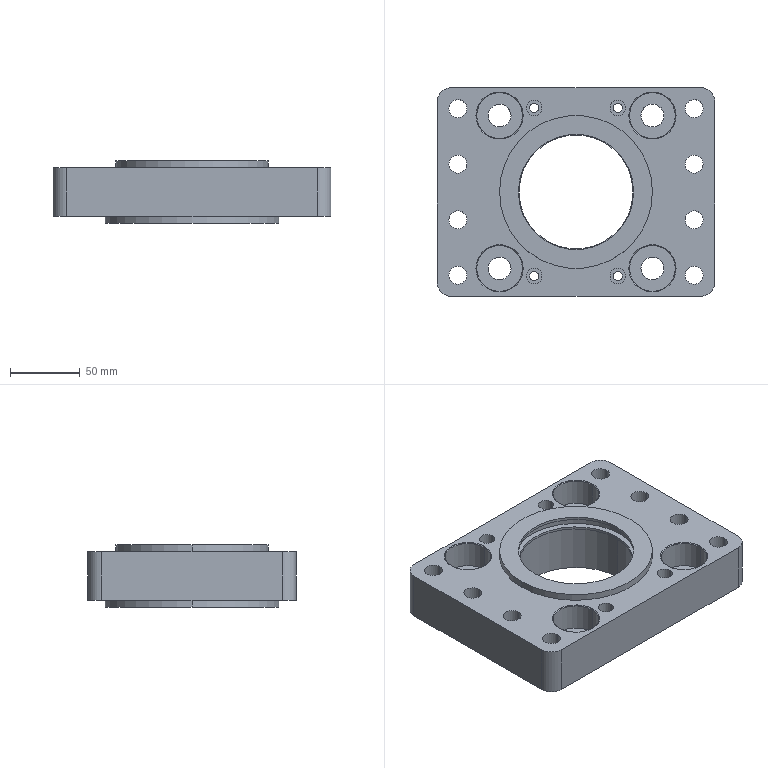Part | SolidWorks | features ICE 9, Chamfer 1, Extrusion 1 | 1 solid | 91 faces | box 200 x 150 x 45 mm | volume 772010 mm3 | cylinder 38 | spline 26 | plane 19 | cone 8 | commonest cylinder face diameters 6.6 x8 11 x8 33 x8 16.5 x2 82 x2 83 x2